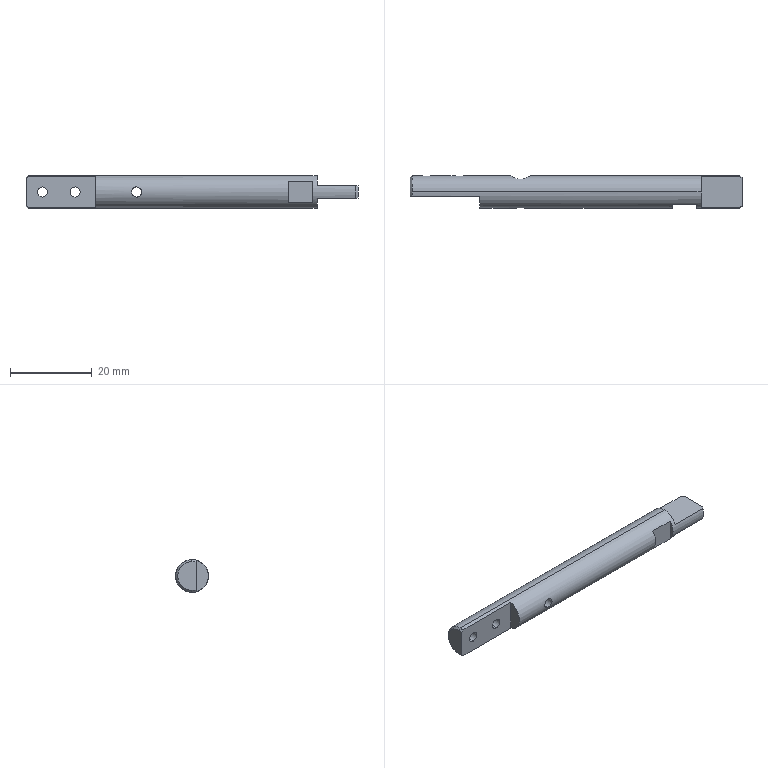Part | STEP file | 0246_205_Rod | 1 solid | 27 faces | box 81 x 8 x 8 mm | volume 3387 mm3 | plane 12 | cylinder 10 | cone 5 | commonest cylinder face diameters 2.5 x6 5 x2 8 x2